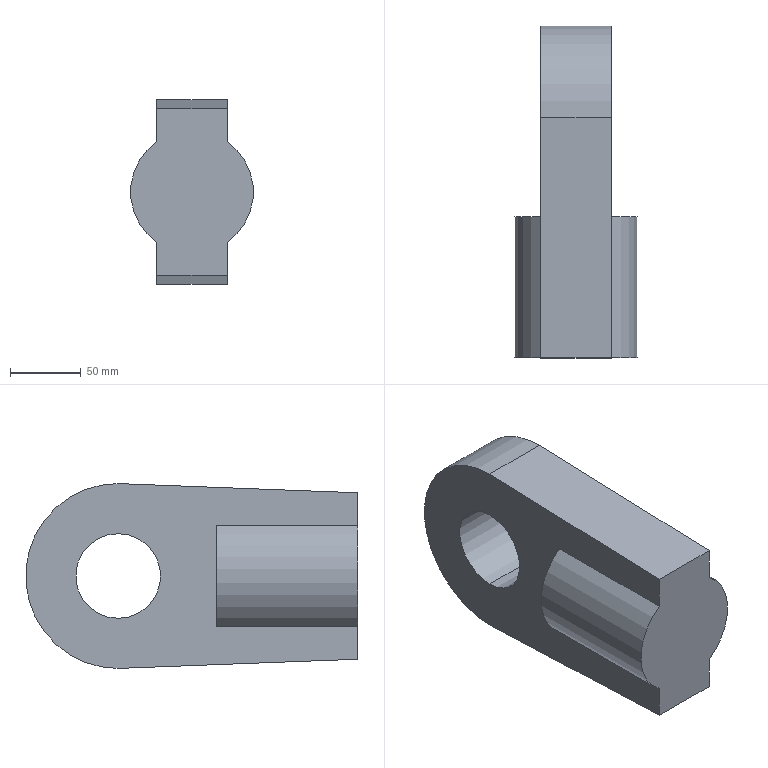Part | SolidWorks | features Extrusion 1, ICE 1 | 1 solid | 12 faces | box 87 x 235.5 x 131 mm | volume 1438602 mm3 | plane 7 | cylinder 5 | commonest cylinder face diameters 60 x2 87 x2 131 x1
STEP:
#1=CARTESIAN_POINT('',(25.,170.,30.));
#2=VERTEX_POINT('',#1);
#3=CARTESIAN_POINT('',(25.,170.,-30.));
#4=VERTEX_POINT('',#3);
#5=CARTESIAN_POINT('',(25.,170.,0.));
#6=DIRECTION('',(1.,0.,0.));
#7=DIRECTION('',(0.,0.,-1.));
#8=AXIS2_PLACEMENT_3D('',#5,#6,#7);
#9=CIRCLE('',#8,30.);
#10=EDGE_CURVE('',#2,#4,#9,.T.);
#11=ORIENTED_EDGE('',*,*,#10,.T.);
#12=CARTESIAN_POINT('',(-25.,170.,-30.));
#13=VERTEX_POINT('',#12);
#14=CARTESIAN_POINT('',(25.,170.,-30.));
#15=DIRECTION('',(-1.,0.,0.));
#16=VECTOR('',#15,1000.);
#17=LINE('',#14,#16);
#18=EDGE_CURVE('',#4,#13,#17,.T.);
#19=ORIENTED_EDGE('',*,*,#18,.T.);
#20=CARTESIAN_POINT('',(-25.,170.,30.));
#21=VERTEX_POINT('',#20);
#22=CARTESIAN_POINT('',(-25.,170.,0.));
#23=DIRECTION('',(1.,0.,0.));
#24=DIRECTION('',(0.,0.,-1.));
#25=AXIS2_PLACEMENT_3D('',#22,#23,#24);
#26=CIRCLE('',#25,30.);
#27=EDGE_CURVE('',#21,#13,#26,.T.);
#28=ORIENTED_EDGE('',*,*,#27,.F.);
#29=CARTESIAN_POINT('',(25.,170.,30.));
#30=DIRECTION('',(-1.,0.,0.));
#31=VECTOR('',#30,1000.);
#32=LINE('',#29,#31);
#33=EDGE_CURVE('',#2,#21,#32,.T.);
#34=ORIENTED_EDGE('',*,*,#33,.F.);
#35=EDGE_LOOP('',(#11,#19,#28,#34));
#36=FACE_OUTER_BOUND('',#35,.T.);
#37=CARTESIAN_POINT('',(25.,170.,0.));
#38=DIRECTION('',(-1.,0.,0.));
#39=DIRECTION('',(0.,0.,1.));
#40=AXIS2_PLACEMENT_3D('',#37,#38,#39);
#41=CYLINDRICAL_SURFACE('',#40,30.);
#42=ADVANCED_FACE('',(#36),#41,.F.);
#43=ORIENTED_EDGE('',*,*,#10,.F.);
#44=CARTESIAN_POINT('',(25.,170.,0.));
#45=DIRECTION('',(1.,0.,0.));
#46=DIRECTION('',(0.,0.,-1.));
#47=AXIS2_PLACEMENT_3D('',#44,#45,#46);
#48=CIRCLE('',#47,30.);
#49=EDGE_CURVE('',#4,#2,#48,.T.);
#50=ORIENTED_EDGE('',*,*,#49,.F.);
#51=EDGE_LOOP('',(#43,#50));
#52=FACE_BOUND('',#51,.T.);
#53=CARTESIAN_POINT('',(25.,0.,35.598));
#54=VERTEX_POINT('',#53);
#55=CARTESIAN_POINT('',(25.,0.,59.));
#56=VERTEX_POINT('',#55);
#57=CARTESIAN_POINT('',(25.,0.,0.));
#58=DIRECTION('',(0.,0.,1.));
#59=VECTOR('',#58,1000.);
#60=LINE('',#57,#59);
#61=EDGE_CURVE('',#54,#56,#60,.T.);
#62=ORIENTED_EDGE('',*,*,#61,.F.);
#63=CARTESIAN_POINT('',(25.,100.,35.598));
#64=VERTEX_POINT('',#63);
#65=CARTESIAN_POINT('',(25.,100.,35.598));
#66=DIRECTION('',(0.,1.,0.));
#67=VECTOR('',#66,1000.);
#68=LINE('',#65,#67);
#69=EDGE_CURVE('',#54,#64,#68,.T.);
#70=ORIENTED_EDGE('',*,*,#69,.T.);
#71=CARTESIAN_POINT('',(25.,100.,-35.598));
#72=VERTEX_POINT('',#71);
#73=CARTESIAN_POINT('',(25.,100.,0.));
#74=DIRECTION('',(0.,0.,1.));
#75=VECTOR('',#74,1000.);
#76=LINE('',#73,#75);
#77=EDGE_CURVE('',#72,#64,#76,.T.);
#78=ORIENTED_EDGE('',*,*,#77,.F.);
#79=CARTESIAN_POINT('',(25.,0.,-35.598));
#80=VERTEX_POINT('',#79);
#81=CARTESIAN_POINT('',(25.,100.,-35.598));
#82=DIRECTION('',(0.,-1.,0.));
#83=VECTOR('',#82,1000.);
#84=LINE('',#81,#83);
#85=EDGE_CURVE('',#72,#80,#84,.T.);
#86=ORIENTED_EDGE('',*,*,#85,.T.);
#87=CARTESIAN_POINT('',(25.,0.,-59.));
#88=VERTEX_POINT('',#87);
#89=CARTESIAN_POINT('',(25.,0.,0.));
#90=DIRECTION('',(0.,0.,1.));
#91=VECTOR('',#90,1000.);
#92=LINE('',#89,#91);
#93=EDGE_CURVE('',#88,#80,#92,.T.);
#94=ORIENTED_EDGE('',*,*,#93,.F.);
#95=CARTESIAN_POINT('',(25.,170.,-65.5));
#96=VERTEX_POINT('',#95);
#97=CARTESIAN_POINT('',(25.,-2.253,-58.914));
#98=DIRECTION('',(0.,0.9993,-0.03821));
#99=VECTOR('',#98,1000.);
#100=LINE('',#97,#99);
#101=EDGE_CURVE('',#88,#96,#100,.T.);
#102=ORIENTED_EDGE('',*,*,#101,.T.);
#103=CARTESIAN_POINT('',(25.,170.,65.5));
#104=VERTEX_POINT('',#103);
#105=CARTESIAN_POINT('',(25.,170.,0.));
#106=DIRECTION('',(1.,0.,0.));
#107=DIRECTION('',(0.,0.,-1.));
#108=AXIS2_PLACEMENT_3D('',#105,#106,#107);
#109=CIRCLE('',#108,65.5);
#110=EDGE_CURVE('',#96,#104,#109,.T.);
#111=ORIENTED_EDGE('',*,*,#110,.T.);
#112=CARTESIAN_POINT('',(25.,-2.253,58.914));
#113=DIRECTION('',(0.,0.9993,0.03821));
#114=VECTOR('',#113,1000.);
#115=LINE('',#112,#114);
#116=EDGE_CURVE('',#56,#104,#115,.T.);
#117=ORIENTED_EDGE('',*,*,#116,.F.);
#118=EDGE_LOOP('',(#62,#70,#78,#86,#94,#102,#111,#117));
#119=FACE_OUTER_BOUND('',#118,.T.);
#120=CARTESIAN_POINT('',(25.,0.,0.));
#121=DIRECTION('',(1.,0.,0.));
#122=DIRECTION('',(0.,0.,-1.));
#123=AXIS2_PLACEMENT_3D('',#120,#121,#122);
#124=PLANE('',#123);
#125=ADVANCED_FACE('',(#52,#119),#124,.T.);
#126=ORIENTED_EDGE('',*,*,#27,.T.);
#127=CARTESIAN_POINT('',(-25.,170.,0.));
#128=DIRECTION('',(1.,0.,0.));
#129=DIRECTION('',(0.,0.,-1.));
#130=AXIS2_PLACEMENT_3D('',#127,#128,#129);
#131=CIRCLE('',#130,30.);
#132=EDGE_CURVE('',#13,#21,#131,.T.);
#133=ORIENTED_EDGE('',*,*,#132,.T.);
#134=EDGE_LOOP('',(#126,#133));
#135=FACE_BOUND('',#134,.T.);
#136=CARTESIAN_POINT('',(-25.,0.,35.598));
#137=VERTEX_POINT('',#136);
#138=CARTESIAN_POINT('',(-25.,100.,35.598));
#139=VERTEX_POINT('',#138);
#140=CARTESIAN_POINT('',(-25.,100.,35.598));
#141=DIRECTION('',(0.,1.,0.));
#142=VECTOR('',#141,1000.);
#143=LINE('',#140,#142);
#144=EDGE_CURVE('',#137,#139,#143,.T.);
#145=ORIENTED_EDGE('',*,*,#144,.F.);
#146=CARTESIAN_POINT('',(-25.,0.,59.));
#147=VERTEX_POINT('',#146);
#148=CARTESIAN_POINT('',(-25.,0.,0.));
#149=DIRECTION('',(0.,0.,1.));
#150=VECTOR('',#149,1000.);
#151=LINE('',#148,#150);
#152=EDGE_CURVE('',#137,#147,#151,.T.);
#153=ORIENTED_EDGE('',*,*,#152,.T.);
#154=CARTESIAN_POINT('',(-25.,170.,65.5));
#155=VERTEX_POINT('',#154);
#156=CARTESIAN_POINT('',(-25.,-2.253,58.914));
#157=DIRECTION('',(0.,0.9993,0.03821));
#158=VECTOR('',#157,1000.);
#159=LINE('',#156,#158);
#160=EDGE_CURVE('',#147,#155,#159,.T.);
#161=ORIENTED_EDGE('',*,*,#160,.T.);
#162=CARTESIAN_POINT('',(-25.,170.,-65.5));
#163=VERTEX_POINT('',#162);
#164=CARTESIAN_POINT('',(-25.,170.,0.));
#165=DIRECTION('',(1.,0.,0.));
#166=DIRECTION('',(0.,0.,-1.));
#167=AXIS2_PLACEMENT_3D('',#164,#165,#166);
#168=CIRCLE('',#167,65.5);
#169=EDGE_CURVE('',#163,#155,#168,.T.);
#170=ORIENTED_EDGE('',*,*,#169,.F.);
#171=CARTESIAN_POINT('',(-25.,0.,-59.));
#172=VERTEX_POINT('',#171);
#173=CARTESIAN_POINT('',(-25.,-2.253,-58.914));
#174=DIRECTION('',(0.,0.9993,-0.03821));
#175=VECTOR('',#174,1000.);
#176=LINE('',#173,#175);
#177=EDGE_CURVE('',#172,#163,#176,.T.);
#178=ORIENTED_EDGE('',*,*,#177,.F.);
#179=CARTESIAN_POINT('',(-25.,0.,-35.598));
#180=VERTEX_POINT('',#179);
#181=CARTESIAN_POINT('',(-25.,0.,0.));
#182=DIRECTION('',(0.,0.,1.));
#183=VECTOR('',#182,1000.);
#184=LINE('',#181,#183);
#185=EDGE_CURVE('',#172,#180,#184,.T.);
#186=ORIENTED_EDGE('',*,*,#185,.T.);
#187=CARTESIAN_POINT('',(-25.,100.,-35.598));
#188=VERTEX_POINT('',#187);
#189=CARTESIAN_POINT('',(-25.,100.,-35.598));
#190=DIRECTION('',(0.,-1.,0.));
#191=VECTOR('',#190,1000.);
#192=LINE('',#189,#191);
#193=EDGE_CURVE('',#188,#180,#192,.T.);
#194=ORIENTED_EDGE('',*,*,#193,.F.);
#195=CARTESIAN_POINT('',(-25.,100.,0.));
#196=DIRECTION('',(0.,0.,1.));
#197=VECTOR('',#196,1000.);
#198=LINE('',#195,#197);
#199=EDGE_CURVE('',#188,#139,#198,.T.);
#200=ORIENTED_EDGE('',*,*,#199,.T.);
#201=EDGE_LOOP('',(#145,#153,#161,#170,#178,#186,#194,#200));
#202=FACE_OUTER_BOUND('',#201,.T.);
#203=CARTESIAN_POINT('',(-25.,0.,0.));
#204=DIRECTION('',(1.,0.,0.));
#205=DIRECTION('',(0.,0.,-1.));
#206=AXIS2_PLACEMENT_3D('',#203,#204,#205);
#207=PLANE('',#206);
#208=ADVANCED_FACE('',(#135,#202),#207,.F.);
#209=ORIENTED_EDGE('',*,*,#93,.T.);
#210=CARTESIAN_POINT('',(0.,0.,0.));
#211=DIRECTION('',(0.,1.,0.));
#212=DIRECTION('',(0.,0.,1.));
#213=AXIS2_PLACEMENT_3D('',#210,#211,#212);
#214=CIRCLE('',#213,43.5);
#215=EDGE_CURVE('',#54,#80,#214,.T.);
#216=ORIENTED_EDGE('',*,*,#215,.F.);
#217=ORIENTED_EDGE('',*,*,#61,.T.);
#218=CARTESIAN_POINT('',(25.,0.,59.));
#219=DIRECTION('',(-1.,0.,0.));
#220=VECTOR('',#219,1000.);
#221=LINE('',#218,#220);
#222=EDGE_CURVE('',#56,#147,#221,.T.);
#223=ORIENTED_EDGE('',*,*,#222,.T.);
#224=ORIENTED_EDGE('',*,*,#152,.F.);
#225=CARTESIAN_POINT('',(0.,0.,0.));
#226=DIRECTION('',(0.,1.,0.));
#227=DIRECTION('',(0.,0.,1.));
#228=AXIS2_PLACEMENT_3D('',#225,#226,#227);
#229=CIRCLE('',#228,43.5);
#230=EDGE_CURVE('',#180,#137,#229,.T.);
#231=ORIENTED_EDGE('',*,*,#230,.F.);
#232=ORIENTED_EDGE('',*,*,#185,.F.);
#233=CARTESIAN_POINT('',(25.,0.,-59.));
#234=DIRECTION('',(-1.,0.,0.));
#235=VECTOR('',#234,1000.);
#236=LINE('',#233,#235);
#237=EDGE_CURVE('',#88,#172,#236,.T.);
#238=ORIENTED_EDGE('',*,*,#237,.F.);
#239=EDGE_LOOP('',(#209,#216,#217,#223,#224,#231,#232,#238));
#240=FACE_OUTER_BOUND('',#239,.T.);
#241=CARTESIAN_POINT('',(25.,0.,0.));
#242=DIRECTION('',(0.,-1.,0.));
#243=DIRECTION('',(0.,0.,-1.));
#244=AXIS2_PLACEMENT_3D('',#241,#242,#243);
#245=PLANE('',#244);
#246=ADVANCED_FACE('',(#240),#245,.T.);
#247=ORIENTED_EDGE('',*,*,#177,.T.);
#248=CARTESIAN_POINT('',(25.,170.,-65.5));
#249=DIRECTION('',(-1.,0.,0.));
#250=VECTOR('',#249,1000.);
#251=LINE('',#248,#250);
#252=EDGE_CURVE('',#96,#163,#251,.T.);
#253=ORIENTED_EDGE('',*,*,#252,.F.);
#254=ORIENTED_EDGE('',*,*,#101,.F.);
#255=ORIENTED_EDGE('',*,*,#237,.T.);
#256=EDGE_LOOP('',(#247,#253,#254,#255));
#257=FACE_OUTER_BOUND('',#256,.T.);
#258=CARTESIAN_POINT('',(25.,-2.253,-58.914));
#259=DIRECTION('',(0.,0.03821,0.9993));
#260=DIRECTION('',(0.,-0.9993,0.03821));
#261=AXIS2_PLACEMENT_3D('',#258,#259,#260);
#262=PLANE('',#261);
#263=ADVANCED_FACE('',(#257),#262,.F.);
#264=ORIENTED_EDGE('',*,*,#169,.T.);
#265=CARTESIAN_POINT('',(25.,170.,65.5));
#266=DIRECTION('',(-1.,0.,0.));
#267=VECTOR('',#266,1000.);
#268=LINE('',#265,#267);
#269=EDGE_CURVE('',#104,#155,#268,.T.);
#270=ORIENTED_EDGE('',*,*,#269,.F.);
#271=ORIENTED_EDGE('',*,*,#110,.F.);
#272=ORIENTED_EDGE('',*,*,#252,.T.);
#273=EDGE_LOOP('',(#264,#270,#271,#272));
#274=FACE_OUTER_BOUND('',#273,.T.);
#275=CARTESIAN_POINT('',(25.,170.,0.));
#276=DIRECTION('',(-1.,0.,0.));
#277=DIRECTION('',(0.,0.,1.));
#278=AXIS2_PLACEMENT_3D('',#275,#276,#277);
#279=CYLINDRICAL_SURFACE('',#278,65.5);
#280=ADVANCED_FACE('',(#274),#279,.T.);
#281=ORIENTED_EDGE('',*,*,#160,.F.);
#282=ORIENTED_EDGE('',*,*,#222,.F.);
#283=ORIENTED_EDGE('',*,*,#116,.T.);
#284=ORIENTED_EDGE('',*,*,#269,.T.);
#285=EDGE_LOOP('',(#281,#282,#283,#284));
#286=FACE_OUTER_BOUND('',#285,.T.);
#287=CARTESIAN_POINT('',(25.,-2.253,58.914));
#288=DIRECTION('',(0.,-0.03821,0.9993));
#289=DIRECTION('',(0.,-0.9993,-0.03821));
#290=AXIS2_PLACEMENT_3D('',#287,#288,#289);
#291=PLANE('',#290);
#292=ADVANCED_FACE('',(#286),#291,.T.);
#293=ORIENTED_EDGE('',*,*,#18,.F.);
#294=ORIENTED_EDGE('',*,*,#49,.T.);
#295=ORIENTED_EDGE('',*,*,#33,.T.);
#296=ORIENTED_EDGE('',*,*,#132,.F.);
#297=EDGE_LOOP('',(#293,#294,#295,#296));
#298=FACE_OUTER_BOUND('',#297,.T.);
#299=CARTESIAN_POINT('',(25.,170.,0.));
#300=DIRECTION('',(-1.,0.,0.));
#301=DIRECTION('',(0.,0.,1.));
#302=AXIS2_PLACEMENT_3D('',#299,#300,#301);
#303=CYLINDRICAL_SURFACE('',#302,30.);
#304=ADVANCED_FACE('',(#298),#303,.F.);
#305=ORIENTED_EDGE('',*,*,#199,.F.);
#306=CARTESIAN_POINT('',(0.,100.,0.));
#307=DIRECTION('',(0.,1.,0.));
#308=DIRECTION('',(0.,0.,1.));
#309=AXIS2_PLACEMENT_3D('',#306,#307,#308);
#310=CIRCLE('',#309,43.5);
#311=EDGE_CURVE('',#188,#139,#310,.T.);
#312=ORIENTED_EDGE('',*,*,#311,.T.);
#313=EDGE_LOOP('',(#305,#312));
#314=FACE_OUTER_BOUND('',#313,.T.);
#315=CARTESIAN_POINT('',(0.,100.,0.));
#316=DIRECTION('',(0.,1.,0.));
#317=DIRECTION('',(0.,0.,1.));
#318=AXIS2_PLACEMENT_3D('',#315,#316,#317);
#319=PLANE('',#318);
#320=ADVANCED_FACE('',(#314),#319,.T.);
#321=ORIENTED_EDGE('',*,*,#230,.T.);
#322=ORIENTED_EDGE('',*,*,#144,.T.);
#323=ORIENTED_EDGE('',*,*,#311,.F.);
#324=ORIENTED_EDGE('',*,*,#193,.T.);
#325=EDGE_LOOP('',(#321,#322,#323,#324));
#326=FACE_OUTER_BOUND('',#325,.T.);
#327=CARTESIAN_POINT('',(0.,100.,0.));
#328=DIRECTION('',(0.,-1.,0.));
#329=DIRECTION('',(0.,0.,-1.));
#330=AXIS2_PLACEMENT_3D('',#327,#328,#329);
#331=CYLINDRICAL_SURFACE('',#330,43.5);
#332=ADVANCED_FACE('',(#326),#331,.T.);
#333=ORIENTED_EDGE('',*,*,#69,.F.);
#334=ORIENTED_EDGE('',*,*,#215,.T.);
#335=ORIENTED_EDGE('',*,*,#85,.F.);
#336=CARTESIAN_POINT('',(0.,100.,0.));
#337=DIRECTION('',(0.,1.,0.));
#338=DIRECTION('',(0.,0.,1.));
#339=AXIS2_PLACEMENT_3D('',#336,#337,#338);
#340=CIRCLE('',#339,43.5);
#341=EDGE_CURVE('',#64,#72,#340,.T.);
#342=ORIENTED_EDGE('',*,*,#341,.F.);
#343=EDGE_LOOP('',(#333,#334,#335,#342));
#344=FACE_OUTER_BOUND('',#343,.T.);
#345=CARTESIAN_POINT('',(0.,100.,0.));
#346=DIRECTION('',(0.,-1.,0.));
#347=DIRECTION('',(0.,0.,-1.));
#348=AXIS2_PLACEMENT_3D('',#345,#346,#347);
#349=CYLINDRICAL_SURFACE('',#348,43.5);
#350=ADVANCED_FACE('',(#344),#349,.T.);
#351=ORIENTED_EDGE('',*,*,#341,.T.);
#352=ORIENTED_EDGE('',*,*,#77,.T.);
#353=EDGE_LOOP('',(#351,#352));
#354=FACE_OUTER_BOUND('',#353,.T.);
#355=CARTESIAN_POINT('',(0.,100.,0.));
#356=DIRECTION('',(0.,1.,0.));
#357=DIRECTION('',(0.,0.,1.));
#358=AXIS2_PLACEMENT_3D('',#355,#356,#357);
#359=PLANE('',#358);
#360=ADVANCED_FACE('',(#354),#359,.T.);
#361=CLOSED_SHELL('',(#42,#125,#208,#246,#263,#280,#292,#304,#320,#332,#350,#360));
#362=MANIFOLD_SOLID_BREP('',#361);
#363=CARTESIAN_POINT('',(0.,0.,0.));
#364=DIRECTION('',(0.,0.,1.));
#365=DIRECTION('',(1.,0.,0.));
#366=AXIS2_PLACEMENT_3D('',#363,#364,#365);
#367=(LENGTH_UNIT()NAMED_UNIT(*)SI_UNIT(.MILLI.,.METRE.));
#368=UNCERTAINTY_MEASURE_WITH_UNIT(LENGTH_MEASURE(0.00001),#367,'','');
#369=(NAMED_UNIT(*)PLANE_ANGLE_UNIT()SI_UNIT($,.RADIAN.));
#370=(NAMED_UNIT(*)SI_UNIT($,.STERADIAN.)SOLID_ANGLE_UNIT());
#371=(GEOMETRIC_REPRESENTATION_CONTEXT(3)GLOBAL_UNCERTAINTY_ASSIGNED_CONTEXT((#368))GLOBAL_UNIT_ASSIGNED_CONTEXT((#367,#369,#370))REPRESENTATION_CONTEXT('',''));
#372=ADVANCED_BREP_SHAPE_REPRESENTATION('',(#362,#366),#371);